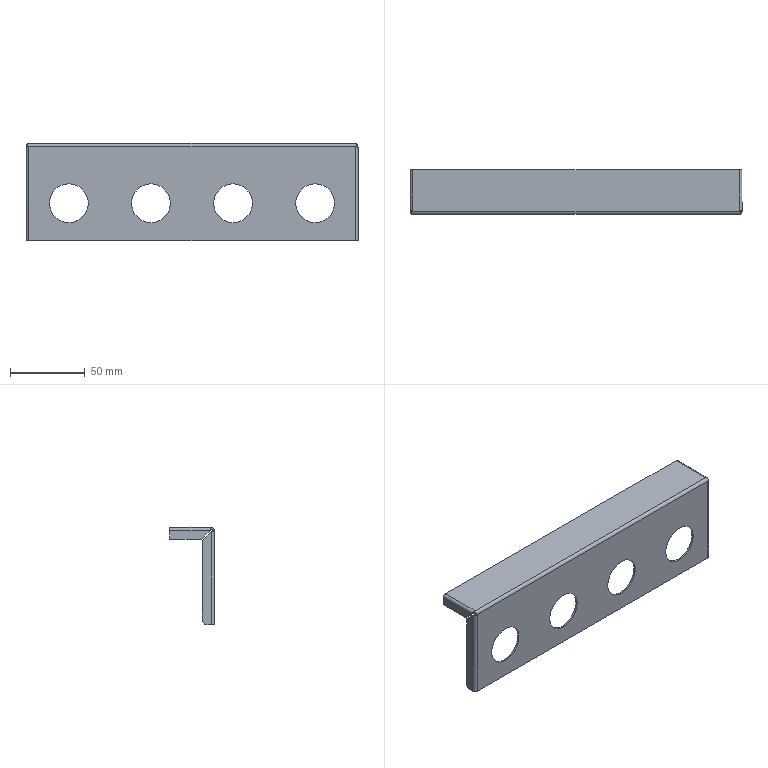Part | SolidWorks | features EdgeFlange 6, Fillet 4, ICE 3, LPattern 2, SMBaseFlange 2, Cut 1, FlatPattern 1, SheetMetal 1 | 1 solid | 60 faces | box 222.4 x 30 x 65 mm | volume 23557 mm3 | plane 36 | cylinder 20 | spline 4 | commonest cylinder face diameters 26 x8 1.6 x5 4 x5 6 x2